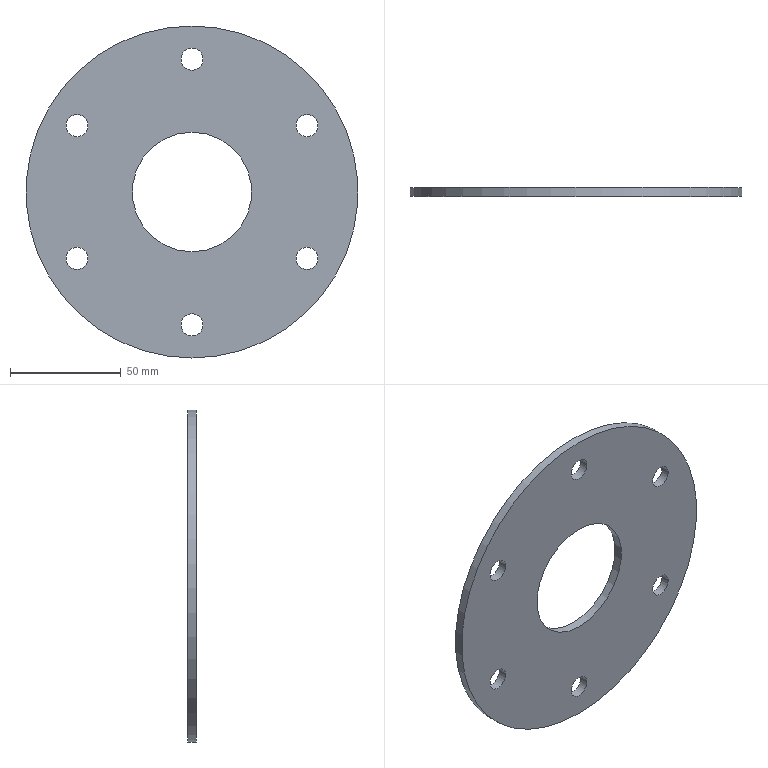Part | STEP file | JBJ-P-1007-03 | 1 solid | 10 faces | box 150 x 4 x 150 mm | volume 59640 mm3 | cylinder 8 | plane 2 | commonest cylinder face diameters 10 x6 54 x1 150 x1
STEP:
#1=CARTESIAN_POINT('',(-51.962,4.,35.));
#2=VERTEX_POINT('',#1);
#3=CARTESIAN_POINT('',(-51.962,4.,30.));
#4=DIRECTION('',(0.,1.,0.));
#5=DIRECTION('',(0.,0.,1.));
#6=AXIS2_PLACEMENT_3D('',#3,#4,#5);
#7=CIRCLE('',#6,5.);
#8=EDGE_CURVE('',#2,#2,#7,.T.);
#9=ORIENTED_EDGE('',*,*,#8,.F.);
#10=EDGE_LOOP('',(#9));
#11=FACE_BOUND('',#10,.T.);
#12=CARTESIAN_POINT('',(51.962,4.,35.));
#13=VERTEX_POINT('',#12);
#14=CARTESIAN_POINT('',(51.962,4.,30.));
#15=DIRECTION('',(0.,1.,0.));
#16=DIRECTION('',(0.,0.,1.));
#17=AXIS2_PLACEMENT_3D('',#14,#15,#16);
#18=CIRCLE('',#17,5.);
#19=EDGE_CURVE('',#13,#13,#18,.T.);
#20=ORIENTED_EDGE('',*,*,#19,.F.);
#21=EDGE_LOOP('',(#20));
#22=FACE_BOUND('',#21,.T.);
#23=CARTESIAN_POINT('',(0.,4.,-55.));
#24=VERTEX_POINT('',#23);
#25=CARTESIAN_POINT('',(0.,4.,-60.));
#26=DIRECTION('',(0.,1.,0.));
#27=DIRECTION('',(0.,0.,1.));
#28=AXIS2_PLACEMENT_3D('',#25,#26,#27);
#29=CIRCLE('',#28,5.);
#30=EDGE_CURVE('',#24,#24,#29,.T.);
#31=ORIENTED_EDGE('',*,*,#30,.F.);
#32=EDGE_LOOP('',(#31));
#33=FACE_BOUND('',#32,.T.);
#34=CARTESIAN_POINT('',(0.,4.,75.));
#35=VERTEX_POINT('',#34);
#36=CARTESIAN_POINT('',(0.,4.,0.));
#37=DIRECTION('',(0.,1.,0.));
#38=DIRECTION('',(0.,0.,1.));
#39=AXIS2_PLACEMENT_3D('',#36,#37,#38);
#40=CIRCLE('',#39,75.);
#41=EDGE_CURVE('',#35,#35,#40,.T.);
#42=ORIENTED_EDGE('',*,*,#41,.T.);
#43=EDGE_LOOP('',(#42));
#44=FACE_OUTER_BOUND('',#43,.T.);
#45=CARTESIAN_POINT('',(0.,4.,27.));
#46=VERTEX_POINT('',#45);
#47=CARTESIAN_POINT('',(0.,4.,0.));
#48=DIRECTION('',(0.,1.,0.));
#49=DIRECTION('',(0.,0.,1.));
#50=AXIS2_PLACEMENT_3D('',#47,#48,#49);
#51=CIRCLE('',#50,27.);
#52=EDGE_CURVE('',#46,#46,#51,.T.);
#53=ORIENTED_EDGE('',*,*,#52,.F.);
#54=EDGE_LOOP('',(#53));
#55=FACE_BOUND('',#54,.T.);
#56=CARTESIAN_POINT('',(51.962,4.,-25.));
#57=VERTEX_POINT('',#56);
#58=CARTESIAN_POINT('',(51.962,4.,-30.));
#59=DIRECTION('',(0.,1.,0.));
#60=DIRECTION('',(0.,0.,1.));
#61=AXIS2_PLACEMENT_3D('',#58,#59,#60);
#62=CIRCLE('',#61,5.);
#63=EDGE_CURVE('',#57,#57,#62,.T.);
#64=ORIENTED_EDGE('',*,*,#63,.F.);
#65=EDGE_LOOP('',(#64));
#66=FACE_BOUND('',#65,.T.);
#67=CARTESIAN_POINT('',(0.,4.,65.));
#68=VERTEX_POINT('',#67);
#69=CARTESIAN_POINT('',(0.,4.,60.));
#70=DIRECTION('',(0.,1.,0.));
#71=DIRECTION('',(0.,0.,1.));
#72=AXIS2_PLACEMENT_3D('',#69,#70,#71);
#73=CIRCLE('',#72,5.);
#74=EDGE_CURVE('',#68,#68,#73,.T.);
#75=ORIENTED_EDGE('',*,*,#74,.F.);
#76=EDGE_LOOP('',(#75));
#77=FACE_BOUND('',#76,.T.);
#78=CARTESIAN_POINT('',(-51.962,4.,-25.));
#79=VERTEX_POINT('',#78);
#80=CARTESIAN_POINT('',(-51.962,4.,-30.));
#81=DIRECTION('',(0.,1.,0.));
#82=DIRECTION('',(0.,0.,1.));
#83=AXIS2_PLACEMENT_3D('',#80,#81,#82);
#84=CIRCLE('',#83,5.);
#85=EDGE_CURVE('',#79,#79,#84,.T.);
#86=ORIENTED_EDGE('',*,*,#85,.F.);
#87=EDGE_LOOP('',(#86));
#88=FACE_BOUND('',#87,.T.);
#89=CARTESIAN_POINT('',(0.,4.,0.));
#90=DIRECTION('',(0.,1.,0.));
#91=DIRECTION('',(0.,0.,1.));
#92=AXIS2_PLACEMENT_3D('',#89,#90,#91);
#93=PLANE('',#92);
#94=ADVANCED_FACE('',(#11,#22,#33,#44,#55,#66,#77,#88),#93,.T.);
#95=CARTESIAN_POINT('',(0.,0.,75.));
#96=VERTEX_POINT('',#95);
#97=CARTESIAN_POINT('',(0.,0.,0.));
#98=DIRECTION('',(0.,1.,0.));
#99=DIRECTION('',(0.,0.,1.));
#100=AXIS2_PLACEMENT_3D('',#97,#98,#99);
#101=CIRCLE('',#100,75.);
#102=EDGE_CURVE('',#96,#96,#101,.T.);
#103=ORIENTED_EDGE('',*,*,#102,.F.);
#104=EDGE_LOOP('',(#103));
#105=FACE_OUTER_BOUND('',#104,.T.);
#106=CARTESIAN_POINT('',(0.,0.,27.));
#107=VERTEX_POINT('',#106);
#108=CARTESIAN_POINT('',(0.,0.,0.));
#109=DIRECTION('',(0.,1.,0.));
#110=DIRECTION('',(0.,0.,1.));
#111=AXIS2_PLACEMENT_3D('',#108,#109,#110);
#112=CIRCLE('',#111,27.);
#113=EDGE_CURVE('',#107,#107,#112,.T.);
#114=ORIENTED_EDGE('',*,*,#113,.T.);
#115=EDGE_LOOP('',(#114));
#116=FACE_BOUND('',#115,.T.);
#117=CARTESIAN_POINT('',(0.,0.,-55.));
#118=VERTEX_POINT('',#117);
#119=CARTESIAN_POINT('',(0.,0.,-60.));
#120=DIRECTION('',(0.,1.,0.));
#121=DIRECTION('',(0.,0.,1.));
#122=AXIS2_PLACEMENT_3D('',#119,#120,#121);
#123=CIRCLE('',#122,5.);
#124=EDGE_CURVE('',#118,#118,#123,.T.);
#125=ORIENTED_EDGE('',*,*,#124,.T.);
#126=EDGE_LOOP('',(#125));
#127=FACE_BOUND('',#126,.T.);
#128=CARTESIAN_POINT('',(51.962,0.,-25.));
#129=VERTEX_POINT('',#128);
#130=CARTESIAN_POINT('',(51.962,0.,-30.));
#131=DIRECTION('',(0.,1.,0.));
#132=DIRECTION('',(0.,0.,1.));
#133=AXIS2_PLACEMENT_3D('',#130,#131,#132);
#134=CIRCLE('',#133,5.);
#135=EDGE_CURVE('',#129,#129,#134,.T.);
#136=ORIENTED_EDGE('',*,*,#135,.T.);
#137=EDGE_LOOP('',(#136));
#138=FACE_BOUND('',#137,.T.);
#139=CARTESIAN_POINT('',(51.962,0.,35.));
#140=VERTEX_POINT('',#139);
#141=CARTESIAN_POINT('',(51.962,0.,30.));
#142=DIRECTION('',(0.,1.,0.));
#143=DIRECTION('',(0.,0.,1.));
#144=AXIS2_PLACEMENT_3D('',#141,#142,#143);
#145=CIRCLE('',#144,5.);
#146=EDGE_CURVE('',#140,#140,#145,.T.);
#147=ORIENTED_EDGE('',*,*,#146,.T.);
#148=EDGE_LOOP('',(#147));
#149=FACE_BOUND('',#148,.T.);
#150=CARTESIAN_POINT('',(0.,0.,65.));
#151=VERTEX_POINT('',#150);
#152=CARTESIAN_POINT('',(0.,0.,60.));
#153=DIRECTION('',(0.,1.,0.));
#154=DIRECTION('',(0.,0.,1.));
#155=AXIS2_PLACEMENT_3D('',#152,#153,#154);
#156=CIRCLE('',#155,5.);
#157=EDGE_CURVE('',#151,#151,#156,.T.);
#158=ORIENTED_EDGE('',*,*,#157,.T.);
#159=EDGE_LOOP('',(#158));
#160=FACE_BOUND('',#159,.T.);
#161=CARTESIAN_POINT('',(-51.962,0.,35.));
#162=VERTEX_POINT('',#161);
#163=CARTESIAN_POINT('',(-51.962,0.,30.));
#164=DIRECTION('',(0.,1.,0.));
#165=DIRECTION('',(0.,0.,1.));
#166=AXIS2_PLACEMENT_3D('',#163,#164,#165);
#167=CIRCLE('',#166,5.);
#168=EDGE_CURVE('',#162,#162,#167,.T.);
#169=ORIENTED_EDGE('',*,*,#168,.T.);
#170=EDGE_LOOP('',(#169));
#171=FACE_BOUND('',#170,.T.);
#172=CARTESIAN_POINT('',(-51.962,0.,-25.));
#173=VERTEX_POINT('',#172);
#174=CARTESIAN_POINT('',(-51.962,0.,-30.));
#175=DIRECTION('',(0.,1.,0.));
#176=DIRECTION('',(0.,0.,1.));
#177=AXIS2_PLACEMENT_3D('',#174,#175,#176);
#178=CIRCLE('',#177,5.);
#179=EDGE_CURVE('',#173,#173,#178,.T.);
#180=ORIENTED_EDGE('',*,*,#179,.T.);
#181=EDGE_LOOP('',(#180));
#182=FACE_BOUND('',#181,.T.);
#183=CARTESIAN_POINT('',(0.,0.,0.));
#184=DIRECTION('',(0.,1.,0.));
#185=DIRECTION('',(0.,0.,1.));
#186=AXIS2_PLACEMENT_3D('',#183,#184,#185);
#187=PLANE('',#186);
#188=ADVANCED_FACE('',(#105,#116,#127,#138,#149,#160,#171,#182),#187,.F.);
#189=ORIENTED_EDGE('',*,*,#41,.F.);
#190=EDGE_LOOP('',(#189));
#191=FACE_OUTER_BOUND('',#190,.T.);
#192=ORIENTED_EDGE('',*,*,#102,.T.);
#193=EDGE_LOOP('',(#192));
#194=FACE_OUTER_BOUND('',#193,.T.);
#195=CARTESIAN_POINT('',(0.,4.,0.));
#196=DIRECTION('',(0.,-1.,0.));
#197=DIRECTION('',(0.,0.,-1.));
#198=AXIS2_PLACEMENT_3D('',#195,#196,#197);
#199=CYLINDRICAL_SURFACE('',#198,75.);
#200=ADVANCED_FACE('',(#191,#194),#199,.T.);
#201=ORIENTED_EDGE('',*,*,#52,.T.);
#202=EDGE_LOOP('',(#201));
#203=FACE_OUTER_BOUND('',#202,.T.);
#204=ORIENTED_EDGE('',*,*,#113,.F.);
#205=EDGE_LOOP('',(#204));
#206=FACE_OUTER_BOUND('',#205,.T.);
#207=CARTESIAN_POINT('',(0.,4.,0.));
#208=DIRECTION('',(0.,-1.,0.));
#209=DIRECTION('',(0.,0.,-1.));
#210=AXIS2_PLACEMENT_3D('',#207,#208,#209);
#211=CYLINDRICAL_SURFACE('',#210,27.);
#212=ADVANCED_FACE('',(#203,#206),#211,.F.);
#213=ORIENTED_EDGE('',*,*,#30,.T.);
#214=EDGE_LOOP('',(#213));
#215=FACE_OUTER_BOUND('',#214,.T.);
#216=ORIENTED_EDGE('',*,*,#124,.F.);
#217=EDGE_LOOP('',(#216));
#218=FACE_OUTER_BOUND('',#217,.T.);
#219=CARTESIAN_POINT('',(0.,4.,-60.));
#220=DIRECTION('',(0.,-1.,0.));
#221=DIRECTION('',(0.,0.,-1.));
#222=AXIS2_PLACEMENT_3D('',#219,#220,#221);
#223=CYLINDRICAL_SURFACE('',#222,5.);
#224=ADVANCED_FACE('',(#215,#218),#223,.F.);
#225=ORIENTED_EDGE('',*,*,#63,.T.);
#226=EDGE_LOOP('',(#225));
#227=FACE_OUTER_BOUND('',#226,.T.);
#228=ORIENTED_EDGE('',*,*,#135,.F.);
#229=EDGE_LOOP('',(#228));
#230=FACE_OUTER_BOUND('',#229,.T.);
#231=CARTESIAN_POINT('',(51.962,4.,-30.));
#232=DIRECTION('',(0.,-1.,0.));
#233=DIRECTION('',(0.,0.,-1.));
#234=AXIS2_PLACEMENT_3D('',#231,#232,#233);
#235=CYLINDRICAL_SURFACE('',#234,5.);
#236=ADVANCED_FACE('',(#227,#230),#235,.F.);
#237=ORIENTED_EDGE('',*,*,#19,.T.);
#238=EDGE_LOOP('',(#237));
#239=FACE_OUTER_BOUND('',#238,.T.);
#240=ORIENTED_EDGE('',*,*,#146,.F.);
#241=EDGE_LOOP('',(#240));
#242=FACE_OUTER_BOUND('',#241,.T.);
#243=CARTESIAN_POINT('',(51.962,4.,30.));
#244=DIRECTION('',(0.,-1.,0.));
#245=DIRECTION('',(0.,0.,-1.));
#246=AXIS2_PLACEMENT_3D('',#243,#244,#245);
#247=CYLINDRICAL_SURFACE('',#246,5.);
#248=ADVANCED_FACE('',(#239,#242),#247,.F.);
#249=ORIENTED_EDGE('',*,*,#74,.T.);
#250=EDGE_LOOP('',(#249));
#251=FACE_OUTER_BOUND('',#250,.T.);
#252=ORIENTED_EDGE('',*,*,#157,.F.);
#253=EDGE_LOOP('',(#252));
#254=FACE_OUTER_BOUND('',#253,.T.);
#255=CARTESIAN_POINT('',(0.,4.,60.));
#256=DIRECTION('',(0.,-1.,0.));
#257=DIRECTION('',(0.,0.,-1.));
#258=AXIS2_PLACEMENT_3D('',#255,#256,#257);
#259=CYLINDRICAL_SURFACE('',#258,5.);
#260=ADVANCED_FACE('',(#251,#254),#259,.F.);
#261=ORIENTED_EDGE('',*,*,#8,.T.);
#262=EDGE_LOOP('',(#261));
#263=FACE_OUTER_BOUND('',#262,.T.);
#264=ORIENTED_EDGE('',*,*,#168,.F.);
#265=EDGE_LOOP('',(#264));
#266=FACE_OUTER_BOUND('',#265,.T.);
#267=CARTESIAN_POINT('',(-51.962,4.,30.));
#268=DIRECTION('',(0.,-1.,0.));
#269=DIRECTION('',(0.,0.,-1.));
#270=AXIS2_PLACEMENT_3D('',#267,#268,#269);
#271=CYLINDRICAL_SURFACE('',#270,5.);
#272=ADVANCED_FACE('',(#263,#266),#271,.F.);
#273=ORIENTED_EDGE('',*,*,#85,.T.);
#274=EDGE_LOOP('',(#273));
#275=FACE_OUTER_BOUND('',#274,.T.);
#276=ORIENTED_EDGE('',*,*,#179,.F.);
#277=EDGE_LOOP('',(#276));
#278=FACE_OUTER_BOUND('',#277,.T.);
#279=CARTESIAN_POINT('',(-51.962,4.,-30.));
#280=DIRECTION('',(0.,-1.,0.));
#281=DIRECTION('',(0.,0.,-1.));
#282=AXIS2_PLACEMENT_3D('',#279,#280,#281);
#283=CYLINDRICAL_SURFACE('',#282,5.);
#284=ADVANCED_FACE('',(#275,#278),#283,.F.);
#285=CLOSED_SHELL('',(#94,#188,#200,#212,#224,#236,#248,#260,#272,#284));
#286=MANIFOLD_SOLID_BREP('',#285);
#287=CARTESIAN_POINT('',(0.,0.,0.));
#288=DIRECTION('',(0.,0.,1.));
#289=DIRECTION('',(1.,0.,0.));
#290=AXIS2_PLACEMENT_3D('',#287,#288,#289);
#291=(LENGTH_UNIT()NAMED_UNIT(*)SI_UNIT(.MILLI.,.METRE.));
#292=UNCERTAINTY_MEASURE_WITH_UNIT(LENGTH_MEASURE(0.00001),#291,'','');
#293=(NAMED_UNIT(*)PLANE_ANGLE_UNIT()SI_UNIT($,.RADIAN.));
#294=(NAMED_UNIT(*)SI_UNIT($,.STERADIAN.)SOLID_ANGLE_UNIT());
#295=(GEOMETRIC_REPRESENTATION_CONTEXT(3)GLOBAL_UNCERTAINTY_ASSIGNED_CONTEXT((#292))GLOBAL_UNIT_ASSIGNED_CONTEXT((#291,#293,#294))REPRESENTATION_CONTEXT('',''));
#296=ADVANCED_BREP_SHAPE_REPRESENTATION('',(#286,#290),#295);